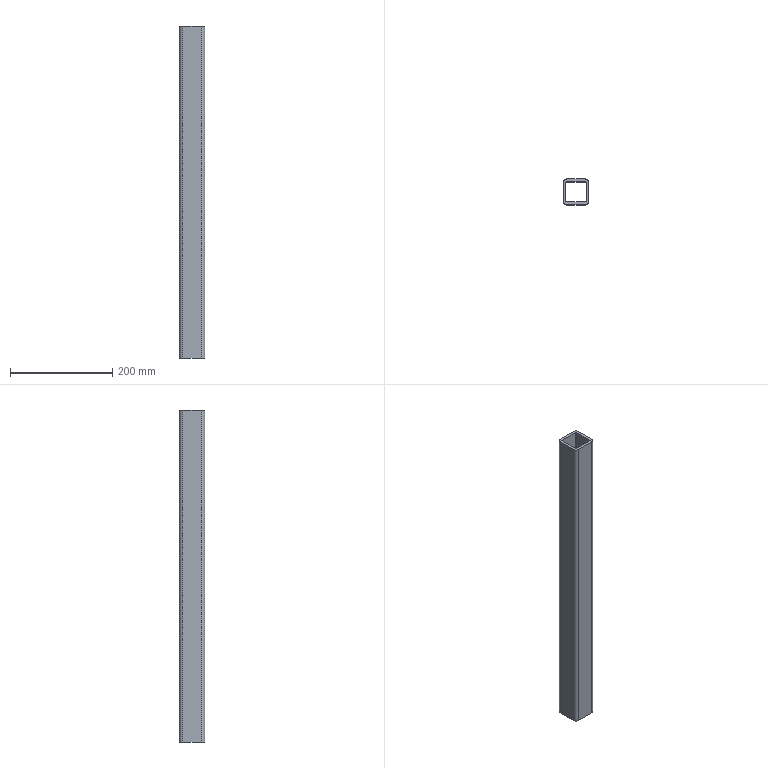Part | NX | 1 solid | 18 faces | box 50 x 50 x 650 mm | volume 559892 mm3 | plane 10 | cylinder 8 | commonest cylinder face diameters 4 x4 14 x4
STEP:
#1=CARTESIAN_POINT('',(-895.,838.,325.));
#2=VERTEX_POINT('',#1);
#3=CARTESIAN_POINT('',(-895.,838.,-325.));
#4=VERTEX_POINT('',#3);
#5=CARTESIAN_POINT('',(-895.,838.,350.));
#6=DIRECTION('',(0.,0.,-1.));
#7=VECTOR('',#6,1000.);
#8=LINE('',#5,#7);
#9=EDGE_CURVE('',#2,#4,#8,.T.);
#10=ORIENTED_EDGE('',*,*,#9,.T.);
#11=CARTESIAN_POINT('',(-895.,874.,-325.));
#12=VERTEX_POINT('',#11);
#13=CARTESIAN_POINT('',(-895.,838.,-325.));
#14=DIRECTION('',(0.,1.,0.));
#15=VECTOR('',#14,1000.);
#16=LINE('',#13,#15);
#17=EDGE_CURVE('',#4,#12,#16,.T.);
#18=ORIENTED_EDGE('',*,*,#17,.T.);
#19=CARTESIAN_POINT('',(-895.,874.,325.));
#20=VERTEX_POINT('',#19);
#21=CARTESIAN_POINT('',(-895.,874.,350.));
#22=DIRECTION('',(0.,0.,-1.));
#23=VECTOR('',#22,1000.);
#24=LINE('',#21,#23);
#25=EDGE_CURVE('',#20,#12,#24,.T.);
#26=ORIENTED_EDGE('',*,*,#25,.F.);
#27=CARTESIAN_POINT('',(-895.,838.,325.));
#28=DIRECTION('',(0.,-1.,0.));
#29=VECTOR('',#28,1000.);
#30=LINE('',#27,#29);
#31=EDGE_CURVE('',#20,#2,#30,.T.);
#32=ORIENTED_EDGE('',*,*,#31,.T.);
#33=EDGE_LOOP('',(#10,#18,#26,#32));
#34=FACE_BOUND('',#33,.T.);
#35=CARTESIAN_POINT('',(-895.,838.,350.));
#36=DIRECTION('',(1.,0.,0.));
#37=DIRECTION('',(0.,1.,0.));
#38=AXIS2_PLACEMENT_3D('',#35,#36,#37);
#39=PLANE('',#38);
#40=ADVANCED_FACE('',(#34),#39,.T.);
#41=CARTESIAN_POINT('',(-893.,836.,325.));
#42=VERTEX_POINT('',#41);
#43=CARTESIAN_POINT('',(-893.,836.,-325.));
#44=VERTEX_POINT('',#43);
#45=CARTESIAN_POINT('',(-893.,836.,350.));
#46=DIRECTION('',(0.,0.,-1.));
#47=VECTOR('',#46,1000.);
#48=LINE('',#45,#47);
#49=EDGE_CURVE('',#42,#44,#48,.T.);
#50=ORIENTED_EDGE('',*,*,#49,.T.);
#51=CARTESIAN_POINT('',(-893.,838.,-325.));
#52=DIRECTION('',(0.,0.,-1.));
#53=DIRECTION('',(0.,1.,0.));
#54=AXIS2_PLACEMENT_3D('',#51,#52,#53);
#55=CIRCLE('',#54,2.);
#56=EDGE_CURVE('',#44,#4,#55,.T.);
#57=ORIENTED_EDGE('',*,*,#56,.T.);
#58=ORIENTED_EDGE('',*,*,#9,.F.);
#59=CARTESIAN_POINT('',(-893.,838.,325.));
#60=DIRECTION('',(0.,0.,1.));
#61=DIRECTION('',(0.,-1.,0.));
#62=AXIS2_PLACEMENT_3D('',#59,#60,#61);
#63=CIRCLE('',#62,2.);
#64=EDGE_CURVE('',#2,#42,#63,.T.);
#65=ORIENTED_EDGE('',*,*,#64,.T.);
#66=EDGE_LOOP('',(#50,#57,#58,#65));
#67=FACE_BOUND('',#66,.T.);
#68=CARTESIAN_POINT('',(-893.,838.,350.));
#69=DIRECTION('',(0.,0.,-1.));
#70=DIRECTION('',(-1.,0.,0.));
#71=AXIS2_PLACEMENT_3D('',#68,#69,#70);
#72=CYLINDRICAL_SURFACE('',#71,2.);
#73=ADVANCED_FACE('',(#67),#72,.F.);
#74=CARTESIAN_POINT('',(-857.,836.,325.));
#75=VERTEX_POINT('',#74);
#76=CARTESIAN_POINT('',(-857.,836.,-325.));
#77=VERTEX_POINT('',#76);
#78=CARTESIAN_POINT('',(-857.,836.,350.));
#79=DIRECTION('',(0.,0.,-1.));
#80=VECTOR('',#79,1000.);
#81=LINE('',#78,#80);
#82=EDGE_CURVE('',#75,#77,#81,.T.);
#83=ORIENTED_EDGE('',*,*,#82,.T.);
#84=CARTESIAN_POINT('',(-893.,836.,-325.));
#85=DIRECTION('',(-1.,0.,0.));
#86=VECTOR('',#85,1000.);
#87=LINE('',#84,#86);
#88=EDGE_CURVE('',#77,#44,#87,.T.);
#89=ORIENTED_EDGE('',*,*,#88,.T.);
#90=ORIENTED_EDGE('',*,*,#49,.F.);
#91=CARTESIAN_POINT('',(-893.,836.,325.));
#92=DIRECTION('',(1.,0.,0.));
#93=VECTOR('',#92,1000.);
#94=LINE('',#91,#93);
#95=EDGE_CURVE('',#42,#75,#94,.T.);
#96=ORIENTED_EDGE('',*,*,#95,.T.);
#97=EDGE_LOOP('',(#83,#89,#90,#96));
#98=FACE_BOUND('',#97,.T.);
#99=CARTESIAN_POINT('',(-893.,836.,350.));
#100=DIRECTION('',(0.,1.,0.));
#101=DIRECTION('',(-1.,0.,0.));
#102=AXIS2_PLACEMENT_3D('',#99,#100,#101);
#103=PLANE('',#102);
#104=ADVANCED_FACE('',(#98),#103,.T.);
#105=CARTESIAN_POINT('',(-855.,838.,325.));
#106=VERTEX_POINT('',#105);
#107=CARTESIAN_POINT('',(-855.,838.,-325.));
#108=VERTEX_POINT('',#107);
#109=CARTESIAN_POINT('',(-855.,838.,350.));
#110=DIRECTION('',(0.,0.,-1.));
#111=VECTOR('',#110,1000.);
#112=LINE('',#109,#111);
#113=EDGE_CURVE('',#106,#108,#112,.T.);
#114=ORIENTED_EDGE('',*,*,#113,.T.);
#115=CARTESIAN_POINT('',(-857.,838.,-325.));
#116=DIRECTION('',(0.,0.,-1.));
#117=DIRECTION('',(0.,1.,0.));
#118=AXIS2_PLACEMENT_3D('',#115,#116,#117);
#119=CIRCLE('',#118,2.);
#120=EDGE_CURVE('',#108,#77,#119,.T.);
#121=ORIENTED_EDGE('',*,*,#120,.T.);
#122=ORIENTED_EDGE('',*,*,#82,.F.);
#123=CARTESIAN_POINT('',(-857.,838.,325.));
#124=DIRECTION('',(0.,0.,1.));
#125=DIRECTION('',(0.,-1.,0.));
#126=AXIS2_PLACEMENT_3D('',#123,#124,#125);
#127=CIRCLE('',#126,2.);
#128=EDGE_CURVE('',#75,#106,#127,.T.);
#129=ORIENTED_EDGE('',*,*,#128,.T.);
#130=EDGE_LOOP('',(#114,#121,#122,#129));
#131=FACE_BOUND('',#130,.T.);
#132=CARTESIAN_POINT('',(-857.,838.,350.));
#133=DIRECTION('',(0.,0.,-1.));
#134=DIRECTION('',(-1.,0.,0.));
#135=AXIS2_PLACEMENT_3D('',#132,#133,#134);
#136=CYLINDRICAL_SURFACE('',#135,2.);
#137=ADVANCED_FACE('',(#131),#136,.F.);
#138=CARTESIAN_POINT('',(-855.,874.,325.));
#139=VERTEX_POINT('',#138);
#140=CARTESIAN_POINT('',(-855.,874.,-325.));
#141=VERTEX_POINT('',#140);
#142=CARTESIAN_POINT('',(-855.,874.,350.));
#143=DIRECTION('',(0.,0.,-1.));
#144=VECTOR('',#143,1000.);
#145=LINE('',#142,#144);
#146=EDGE_CURVE('',#139,#141,#145,.T.);
#147=ORIENTED_EDGE('',*,*,#146,.T.);
#148=CARTESIAN_POINT('',(-855.,874.,-325.));
#149=DIRECTION('',(0.,-1.,0.));
#150=VECTOR('',#149,1000.);
#151=LINE('',#148,#150);
#152=EDGE_CURVE('',#141,#108,#151,.T.);
#153=ORIENTED_EDGE('',*,*,#152,.T.);
#154=ORIENTED_EDGE('',*,*,#113,.F.);
#155=CARTESIAN_POINT('',(-855.,874.,325.));
#156=DIRECTION('',(0.,1.,0.));
#157=VECTOR('',#156,1000.);
#158=LINE('',#155,#157);
#159=EDGE_CURVE('',#106,#139,#158,.T.);
#160=ORIENTED_EDGE('',*,*,#159,.T.);
#161=EDGE_LOOP('',(#147,#153,#154,#160));
#162=FACE_BOUND('',#161,.T.);
#163=CARTESIAN_POINT('',(-855.,874.,350.));
#164=DIRECTION('',(-1.,0.,0.));
#165=DIRECTION('',(0.,-1.,0.));
#166=AXIS2_PLACEMENT_3D('',#163,#164,#165);
#167=PLANE('',#166);
#168=ADVANCED_FACE('',(#162),#167,.T.);
#169=CARTESIAN_POINT('',(-857.,876.,325.));
#170=VERTEX_POINT('',#169);
#171=CARTESIAN_POINT('',(-857.,876.,-325.));
#172=VERTEX_POINT('',#171);
#173=CARTESIAN_POINT('',(-857.,876.,350.));
#174=DIRECTION('',(0.,0.,-1.));
#175=VECTOR('',#174,1000.);
#176=LINE('',#173,#175);
#177=EDGE_CURVE('',#170,#172,#176,.T.);
#178=ORIENTED_EDGE('',*,*,#177,.T.);
#179=CARTESIAN_POINT('',(-857.,874.,-325.));
#180=DIRECTION('',(0.,0.,-1.));
#181=DIRECTION('',(0.,1.,0.));
#182=AXIS2_PLACEMENT_3D('',#179,#180,#181);
#183=CIRCLE('',#182,2.);
#184=EDGE_CURVE('',#172,#141,#183,.T.);
#185=ORIENTED_EDGE('',*,*,#184,.T.);
#186=ORIENTED_EDGE('',*,*,#146,.F.);
#187=CARTESIAN_POINT('',(-857.,874.,325.));
#188=DIRECTION('',(0.,0.,1.));
#189=DIRECTION('',(0.,-1.,0.));
#190=AXIS2_PLACEMENT_3D('',#187,#188,#189);
#191=CIRCLE('',#190,2.);
#192=EDGE_CURVE('',#139,#170,#191,.T.);
#193=ORIENTED_EDGE('',*,*,#192,.T.);
#194=EDGE_LOOP('',(#178,#185,#186,#193));
#195=FACE_BOUND('',#194,.T.);
#196=CARTESIAN_POINT('',(-857.,874.,350.));
#197=DIRECTION('',(0.,0.,-1.));
#198=DIRECTION('',(-1.,0.,0.));
#199=AXIS2_PLACEMENT_3D('',#196,#197,#198);
#200=CYLINDRICAL_SURFACE('',#199,2.);
#201=ADVANCED_FACE('',(#195),#200,.F.);
#202=CARTESIAN_POINT('',(-893.,876.,325.));
#203=VERTEX_POINT('',#202);
#204=CARTESIAN_POINT('',(-893.,876.,-325.));
#205=VERTEX_POINT('',#204);
#206=CARTESIAN_POINT('',(-893.,876.,350.));
#207=DIRECTION('',(0.,0.,-1.));
#208=VECTOR('',#207,1000.);
#209=LINE('',#206,#208);
#210=EDGE_CURVE('',#203,#205,#209,.T.);
#211=ORIENTED_EDGE('',*,*,#210,.T.);
#212=CARTESIAN_POINT('',(-857.,876.,-325.));
#213=DIRECTION('',(1.,0.,0.));
#214=VECTOR('',#213,1000.);
#215=LINE('',#212,#214);
#216=EDGE_CURVE('',#205,#172,#215,.T.);
#217=ORIENTED_EDGE('',*,*,#216,.T.);
#218=ORIENTED_EDGE('',*,*,#177,.F.);
#219=CARTESIAN_POINT('',(-857.,876.,325.));
#220=DIRECTION('',(-1.,0.,0.));
#221=VECTOR('',#220,1000.);
#222=LINE('',#219,#221);
#223=EDGE_CURVE('',#170,#203,#222,.T.);
#224=ORIENTED_EDGE('',*,*,#223,.T.);
#225=EDGE_LOOP('',(#211,#217,#218,#224));
#226=FACE_BOUND('',#225,.T.);
#227=CARTESIAN_POINT('',(-857.,876.,350.));
#228=DIRECTION('',(0.,-1.,0.));
#229=DIRECTION('',(1.,0.,0.));
#230=AXIS2_PLACEMENT_3D('',#227,#228,#229);
#231=PLANE('',#230);
#232=ADVANCED_FACE('',(#226),#231,.T.);
#233=ORIENTED_EDGE('',*,*,#25,.T.);
#234=CARTESIAN_POINT('',(-893.,874.,-325.));
#235=DIRECTION('',(0.,0.,-1.));
#236=DIRECTION('',(0.,1.,0.));
#237=AXIS2_PLACEMENT_3D('',#234,#235,#236);
#238=CIRCLE('',#237,2.);
#239=EDGE_CURVE('',#12,#205,#238,.T.);
#240=ORIENTED_EDGE('',*,*,#239,.T.);
#241=ORIENTED_EDGE('',*,*,#210,.F.);
#242=CARTESIAN_POINT('',(-893.,874.,325.));
#243=DIRECTION('',(0.,0.,1.));
#244=DIRECTION('',(0.,-1.,0.));
#245=AXIS2_PLACEMENT_3D('',#242,#243,#244);
#246=CIRCLE('',#245,2.);
#247=EDGE_CURVE('',#203,#20,#246,.T.);
#248=ORIENTED_EDGE('',*,*,#247,.T.);
#249=EDGE_LOOP('',(#233,#240,#241,#248));
#250=FACE_BOUND('',#249,.T.);
#251=CARTESIAN_POINT('',(-893.,874.,350.));
#252=DIRECTION('',(0.,0.,-1.));
#253=DIRECTION('',(-1.,0.,0.));
#254=AXIS2_PLACEMENT_3D('',#251,#252,#253);
#255=CYLINDRICAL_SURFACE('',#254,2.);
#256=ADVANCED_FACE('',(#250),#255,.F.);
#257=CARTESIAN_POINT('',(-850.,874.,-325.));
#258=VERTEX_POINT('',#257);
#259=CARTESIAN_POINT('',(-850.,838.,-325.));
#260=VERTEX_POINT('',#259);
#261=CARTESIAN_POINT('',(-850.,874.,-325.));
#262=DIRECTION('',(0.,-1.,0.));
#263=VECTOR('',#262,1000.);
#264=LINE('',#261,#263);
#265=EDGE_CURVE('',#258,#260,#264,.T.);
#266=ORIENTED_EDGE('',*,*,#265,.F.);
#267=CARTESIAN_POINT('',(-850.,874.,325.));
#268=VERTEX_POINT('',#267);
#269=CARTESIAN_POINT('',(-850.,874.,350.));
#270=DIRECTION('',(0.,0.,-1.));
#271=VECTOR('',#270,1000.);
#272=LINE('',#269,#271);
#273=EDGE_CURVE('',#268,#258,#272,.T.);
#274=ORIENTED_EDGE('',*,*,#273,.F.);
#275=CARTESIAN_POINT('',(-850.,838.,325.));
#276=VERTEX_POINT('',#275);
#277=CARTESIAN_POINT('',(-850.,874.,325.));
#278=DIRECTION('',(0.,1.,0.));
#279=VECTOR('',#278,1000.);
#280=LINE('',#277,#279);
#281=EDGE_CURVE('',#276,#268,#280,.T.);
#282=ORIENTED_EDGE('',*,*,#281,.F.);
#283=CARTESIAN_POINT('',(-850.,838.,350.));
#284=DIRECTION('',(0.,0.,-1.));
#285=VECTOR('',#284,1000.);
#286=LINE('',#283,#285);
#287=EDGE_CURVE('',#276,#260,#286,.T.);
#288=ORIENTED_EDGE('',*,*,#287,.T.);
#289=EDGE_LOOP('',(#266,#274,#282,#288));
#290=FACE_BOUND('',#289,.T.);
#291=CARTESIAN_POINT('',(-850.,874.,350.));
#292=DIRECTION('',(-1.,0.,0.));
#293=DIRECTION('',(0.,-1.,0.));
#294=AXIS2_PLACEMENT_3D('',#291,#292,#293);
#295=PLANE('',#294);
#296=ADVANCED_FACE('',(#290),#295,.F.);
#297=CARTESIAN_POINT('',(-857.,831.,-325.));
#298=VERTEX_POINT('',#297);
#299=CARTESIAN_POINT('',(-857.,838.,-325.));
#300=DIRECTION('',(0.,0.,-1.));
#301=DIRECTION('',(0.,1.,0.));
#302=AXIS2_PLACEMENT_3D('',#299,#300,#301);
#303=CIRCLE('',#302,7.);
#304=EDGE_CURVE('',#260,#298,#303,.T.);
#305=ORIENTED_EDGE('',*,*,#304,.F.);
#306=ORIENTED_EDGE('',*,*,#287,.F.);
#307=CARTESIAN_POINT('',(-857.,831.,325.));
#308=VERTEX_POINT('',#307);
#309=CARTESIAN_POINT('',(-857.,838.,325.));
#310=DIRECTION('',(0.,0.,1.));
#311=DIRECTION('',(0.,-1.,0.));
#312=AXIS2_PLACEMENT_3D('',#309,#310,#311);
#313=CIRCLE('',#312,7.);
#314=EDGE_CURVE('',#308,#276,#313,.T.);
#315=ORIENTED_EDGE('',*,*,#314,.F.);
#316=CARTESIAN_POINT('',(-857.,831.,350.));
#317=DIRECTION('',(0.,0.,-1.));
#318=VECTOR('',#317,1000.);
#319=LINE('',#316,#318);
#320=EDGE_CURVE('',#308,#298,#319,.T.);
#321=ORIENTED_EDGE('',*,*,#320,.T.);
#322=EDGE_LOOP('',(#305,#306,#315,#321));
#323=FACE_BOUND('',#322,.T.);
#324=CARTESIAN_POINT('',(-857.,838.,350.));
#325=DIRECTION('',(0.,0.,-1.));
#326=DIRECTION('',(-1.,0.,0.));
#327=AXIS2_PLACEMENT_3D('',#324,#325,#326);
#328=CYLINDRICAL_SURFACE('',#327,7.);
#329=ADVANCED_FACE('',(#323),#328,.T.);
#330=CARTESIAN_POINT('',(-893.,831.,-325.));
#331=VERTEX_POINT('',#330);
#332=CARTESIAN_POINT('',(-975.,831.,-325.));
#333=DIRECTION('',(1.,0.,0.));
#334=VECTOR('',#333,1000.);
#335=LINE('',#332,#334);
#336=EDGE_CURVE('',#331,#298,#335,.T.);
#337=ORIENTED_EDGE('',*,*,#336,.T.);
#338=ORIENTED_EDGE('',*,*,#320,.F.);
#339=CARTESIAN_POINT('',(-893.,831.,325.));
#340=VERTEX_POINT('',#339);
#341=CARTESIAN_POINT('',(-975.,831.,325.));
#342=DIRECTION('',(1.,0.,0.));
#343=VECTOR('',#342,1000.);
#344=LINE('',#341,#343);
#345=EDGE_CURVE('',#340,#308,#344,.T.);
#346=ORIENTED_EDGE('',*,*,#345,.F.);
#347=CARTESIAN_POINT('',(-893.,831.,350.));
#348=DIRECTION('',(0.,0.,-1.));
#349=VECTOR('',#348,1000.);
#350=LINE('',#347,#349);
#351=EDGE_CURVE('',#340,#331,#350,.T.);
#352=ORIENTED_EDGE('',*,*,#351,.T.);
#353=EDGE_LOOP('',(#337,#338,#346,#352));
#354=FACE_BOUND('',#353,.T.);
#355=CARTESIAN_POINT('',(-893.,831.,350.));
#356=DIRECTION('',(0.,1.,0.));
#357=DIRECTION('',(-1.,0.,0.));
#358=AXIS2_PLACEMENT_3D('',#355,#356,#357);
#359=PLANE('',#358);
#360=ADVANCED_FACE('',(#354),#359,.F.);
#361=CARTESIAN_POINT('',(-900.,838.,-325.));
#362=VERTEX_POINT('',#361);
#363=CARTESIAN_POINT('',(-893.,838.,-325.));
#364=DIRECTION('',(0.,0.,-1.));
#365=DIRECTION('',(0.,1.,0.));
#366=AXIS2_PLACEMENT_3D('',#363,#364,#365);
#367=CIRCLE('',#366,7.);
#368=EDGE_CURVE('',#331,#362,#367,.T.);
#369=ORIENTED_EDGE('',*,*,#368,.F.);
#370=ORIENTED_EDGE('',*,*,#351,.F.);
#371=CARTESIAN_POINT('',(-900.,838.,325.));
#372=VERTEX_POINT('',#371);
#373=CARTESIAN_POINT('',(-893.,838.,325.));
#374=DIRECTION('',(0.,0.,1.));
#375=DIRECTION('',(0.,-1.,0.));
#376=AXIS2_PLACEMENT_3D('',#373,#374,#375);
#377=CIRCLE('',#376,7.);
#378=EDGE_CURVE('',#372,#340,#377,.T.);
#379=ORIENTED_EDGE('',*,*,#378,.F.);
#380=CARTESIAN_POINT('',(-900.,838.,350.));
#381=DIRECTION('',(0.,0.,-1.));
#382=VECTOR('',#381,1000.);
#383=LINE('',#380,#382);
#384=EDGE_CURVE('',#372,#362,#383,.T.);
#385=ORIENTED_EDGE('',*,*,#384,.T.);
#386=EDGE_LOOP('',(#369,#370,#379,#385));
#387=FACE_BOUND('',#386,.T.);
#388=CARTESIAN_POINT('',(-893.,838.,350.));
#389=DIRECTION('',(0.,0.,-1.));
#390=DIRECTION('',(-1.,0.,0.));
#391=AXIS2_PLACEMENT_3D('',#388,#389,#390);
#392=CYLINDRICAL_SURFACE('',#391,7.);
#393=ADVANCED_FACE('',(#387),#392,.T.);
#394=CARTESIAN_POINT('',(-900.,874.,-325.));
#395=VERTEX_POINT('',#394);
#396=CARTESIAN_POINT('',(-900.,838.,-325.));
#397=DIRECTION('',(0.,1.,0.));
#398=VECTOR('',#397,1000.);
#399=LINE('',#396,#398);
#400=EDGE_CURVE('',#362,#395,#399,.T.);
#401=ORIENTED_EDGE('',*,*,#400,.F.);
#402=ORIENTED_EDGE('',*,*,#384,.F.);
#403=CARTESIAN_POINT('',(-900.,874.,325.));
#404=VERTEX_POINT('',#403);
#405=CARTESIAN_POINT('',(-900.,838.,325.));
#406=DIRECTION('',(0.,-1.,0.));
#407=VECTOR('',#406,1000.);
#408=LINE('',#405,#407);
#409=EDGE_CURVE('',#404,#372,#408,.T.);
#410=ORIENTED_EDGE('',*,*,#409,.F.);
#411=CARTESIAN_POINT('',(-900.,874.,350.));
#412=DIRECTION('',(0.,0.,-1.));
#413=VECTOR('',#412,1000.);
#414=LINE('',#411,#413);
#415=EDGE_CURVE('',#404,#395,#414,.T.);
#416=ORIENTED_EDGE('',*,*,#415,.T.);
#417=EDGE_LOOP('',(#401,#402,#410,#416));
#418=FACE_BOUND('',#417,.T.);
#419=CARTESIAN_POINT('',(-900.,838.,350.));
#420=DIRECTION('',(1.,0.,0.));
#421=DIRECTION('',(0.,1.,0.));
#422=AXIS2_PLACEMENT_3D('',#419,#420,#421);
#423=PLANE('',#422);
#424=ADVANCED_FACE('',(#418),#423,.F.);
#425=CARTESIAN_POINT('',(-893.,881.,-325.));
#426=VERTEX_POINT('',#425);
#427=CARTESIAN_POINT('',(-893.,874.,-325.));
#428=DIRECTION('',(0.,0.,-1.));
#429=DIRECTION('',(0.,1.,0.));
#430=AXIS2_PLACEMENT_3D('',#427,#428,#429);
#431=CIRCLE('',#430,7.);
#432=EDGE_CURVE('',#395,#426,#431,.T.);
#433=ORIENTED_EDGE('',*,*,#432,.F.);
#434=ORIENTED_EDGE('',*,*,#415,.F.);
#435=CARTESIAN_POINT('',(-893.,881.,325.));
#436=VERTEX_POINT('',#435);
#437=CARTESIAN_POINT('',(-893.,874.,325.));
#438=DIRECTION('',(0.,0.,1.));
#439=DIRECTION('',(0.,-1.,0.));
#440=AXIS2_PLACEMENT_3D('',#437,#438,#439);
#441=CIRCLE('',#440,7.);
#442=EDGE_CURVE('',#436,#404,#441,.T.);
#443=ORIENTED_EDGE('',*,*,#442,.F.);
#444=CARTESIAN_POINT('',(-893.,881.,350.));
#445=DIRECTION('',(0.,0.,-1.));
#446=VECTOR('',#445,1000.);
#447=LINE('',#444,#446);
#448=EDGE_CURVE('',#436,#426,#447,.T.);
#449=ORIENTED_EDGE('',*,*,#448,.T.);
#450=EDGE_LOOP('',(#433,#434,#443,#449));
#451=FACE_BOUND('',#450,.T.);
#452=CARTESIAN_POINT('',(-893.,874.,350.));
#453=DIRECTION('',(0.,0.,-1.));
#454=DIRECTION('',(-1.,0.,0.));
#455=AXIS2_PLACEMENT_3D('',#452,#453,#454);
#456=CYLINDRICAL_SURFACE('',#455,7.);
#457=ADVANCED_FACE('',(#451),#456,.T.);
#458=CARTESIAN_POINT('',(-857.,881.,-325.));
#459=VERTEX_POINT('',#458);
#460=CARTESIAN_POINT('',(-975.,881.,-325.));
#461=DIRECTION('',(1.,0.,0.));
#462=VECTOR('',#461,1000.);
#463=LINE('',#460,#462);
#464=EDGE_CURVE('',#426,#459,#463,.T.);
#465=ORIENTED_EDGE('',*,*,#464,.F.);
#466=ORIENTED_EDGE('',*,*,#448,.F.);
#467=CARTESIAN_POINT('',(-857.,881.,325.));
#468=VERTEX_POINT('',#467);
#469=CARTESIAN_POINT('',(-975.,881.,325.));
#470=DIRECTION('',(1.,0.,0.));
#471=VECTOR('',#470,1000.);
#472=LINE('',#469,#471);
#473=EDGE_CURVE('',#436,#468,#472,.T.);
#474=ORIENTED_EDGE('',*,*,#473,.T.);
#475=CARTESIAN_POINT('',(-857.,881.,350.));
#476=DIRECTION('',(0.,0.,-1.));
#477=VECTOR('',#476,1000.);
#478=LINE('',#475,#477);
#479=EDGE_CURVE('',#468,#459,#478,.T.);
#480=ORIENTED_EDGE('',*,*,#479,.T.);
#481=EDGE_LOOP('',(#465,#466,#474,#480));
#482=FACE_BOUND('',#481,.T.);
#483=CARTESIAN_POINT('',(-857.,881.,350.));
#484=DIRECTION('',(0.,-1.,0.));
#485=DIRECTION('',(1.,0.,0.));
#486=AXIS2_PLACEMENT_3D('',#483,#484,#485);
#487=PLANE('',#486);
#488=ADVANCED_FACE('',(#482),#487,.F.);
#489=CARTESIAN_POINT('',(-857.,874.,-325.));
#490=DIRECTION('',(0.,0.,-1.));
#491=DIRECTION('',(0.,1.,0.));
#492=AXIS2_PLACEMENT_3D('',#489,#490,#491);
#493=CIRCLE('',#492,7.);
#494=EDGE_CURVE('',#459,#258,#493,.T.);
#495=ORIENTED_EDGE('',*,*,#494,.F.);
#496=ORIENTED_EDGE('',*,*,#479,.F.);
#497=CARTESIAN_POINT('',(-857.,874.,325.));
#498=DIRECTION('',(0.,0.,1.));
#499=DIRECTION('',(0.,-1.,0.));
#500=AXIS2_PLACEMENT_3D('',#497,#498,#499);
#501=CIRCLE('',#500,7.);
#502=EDGE_CURVE('',#268,#468,#501,.T.);
#503=ORIENTED_EDGE('',*,*,#502,.F.);
#504=ORIENTED_EDGE('',*,*,#273,.T.);
#505=EDGE_LOOP('',(#495,#496,#503,#504));
#506=FACE_BOUND('',#505,.T.);
#507=CARTESIAN_POINT('',(-857.,874.,350.));
#508=DIRECTION('',(0.,0.,-1.));
#509=DIRECTION('',(-1.,0.,0.));
#510=AXIS2_PLACEMENT_3D('',#507,#508,#509);
#511=CYLINDRICAL_SURFACE('',#510,7.);
#512=ADVANCED_FACE('',(#506),#511,.T.);
#513=ORIENTED_EDGE('',*,*,#223,.F.);
#514=ORIENTED_EDGE('',*,*,#192,.F.);
#515=ORIENTED_EDGE('',*,*,#159,.F.);
#516=ORIENTED_EDGE('',*,*,#128,.F.);
#517=ORIENTED_EDGE('',*,*,#95,.F.);
#518=ORIENTED_EDGE('',*,*,#64,.F.);
#519=ORIENTED_EDGE('',*,*,#31,.F.);
#520=ORIENTED_EDGE('',*,*,#247,.F.);
#521=EDGE_LOOP('',(#513,#514,#515,#516,#517,#518,#519,#520));
#522=FACE_BOUND('',#521,.T.);
#523=ORIENTED_EDGE('',*,*,#442,.T.);
#524=ORIENTED_EDGE('',*,*,#409,.T.);
#525=ORIENTED_EDGE('',*,*,#378,.T.);
#526=ORIENTED_EDGE('',*,*,#345,.T.);
#527=ORIENTED_EDGE('',*,*,#314,.T.);
#528=ORIENTED_EDGE('',*,*,#281,.T.);
#529=ORIENTED_EDGE('',*,*,#502,.T.);
#530=ORIENTED_EDGE('',*,*,#473,.F.);
#531=EDGE_LOOP('',(#523,#524,#525,#526,#527,#528,#529,#530));
#532=FACE_BOUND('',#531,.T.);
#533=CARTESIAN_POINT('',(-975.,838.,325.));
#534=DIRECTION('',(0.,0.,1.));
#535=DIRECTION('',(0.,-1.,0.));
#536=AXIS2_PLACEMENT_3D('',#533,#534,#535);
#537=PLANE('',#536);
#538=ADVANCED_FACE('',(#522,#532),#537,.T.);
#539=ORIENTED_EDGE('',*,*,#56,.F.);
#540=ORIENTED_EDGE('',*,*,#88,.F.);
#541=ORIENTED_EDGE('',*,*,#120,.F.);
#542=ORIENTED_EDGE('',*,*,#152,.F.);
#543=ORIENTED_EDGE('',*,*,#184,.F.);
#544=ORIENTED_EDGE('',*,*,#216,.F.);
#545=ORIENTED_EDGE('',*,*,#239,.F.);
#546=ORIENTED_EDGE('',*,*,#17,.F.);
#547=EDGE_LOOP('',(#539,#540,#541,#542,#543,#544,#545,#546));
#548=FACE_BOUND('',#547,.T.);
#549=ORIENTED_EDGE('',*,*,#368,.T.);
#550=ORIENTED_EDGE('',*,*,#400,.T.);
#551=ORIENTED_EDGE('',*,*,#432,.T.);
#552=ORIENTED_EDGE('',*,*,#464,.T.);
#553=ORIENTED_EDGE('',*,*,#494,.T.);
#554=ORIENTED_EDGE('',*,*,#265,.T.);
#555=ORIENTED_EDGE('',*,*,#304,.T.);
#556=ORIENTED_EDGE('',*,*,#336,.F.);
#557=EDGE_LOOP('',(#549,#550,#551,#552,#553,#554,#555,#556));
#558=FACE_BOUND('',#557,.T.);
#559=CARTESIAN_POINT('',(-975.,874.,-325.));
#560=DIRECTION('',(0.,0.,-1.));
#561=DIRECTION('',(0.,1.,0.));
#562=AXIS2_PLACEMENT_3D('',#559,#560,#561);
#563=PLANE('',#562);
#564=ADVANCED_FACE('',(#548,#558),#563,.T.);
#565=CLOSED_SHELL('',(#40,#73,#104,#137,#168,#201,#232,#256,#296,#329,#360,#393,#424,#457,#488,#512,#538,#564));
#566=MANIFOLD_SOLID_BREP('',#565);
#567=(LENGTH_UNIT()NAMED_UNIT(*)SI_UNIT(.MILLI.,.METRE.));
#568=UNCERTAINTY_MEASURE_WITH_UNIT(LENGTH_MEASURE(0.00001),#567,'','');
#569=(NAMED_UNIT(*)PLANE_ANGLE_UNIT()SI_UNIT($,.RADIAN.));
#570=(NAMED_UNIT(*)SI_UNIT($,.STERADIAN.)SOLID_ANGLE_UNIT());
#571=(GEOMETRIC_REPRESENTATION_CONTEXT(3)GLOBAL_UNCERTAINTY_ASSIGNED_CONTEXT((#568))GLOBAL_UNIT_ASSIGNED_CONTEXT((#567,#569,#570))REPRESENTATION_CONTEXT('',''));
#572=ADVANCED_BREP_SHAPE_REPRESENTATION('',(#566),#571);